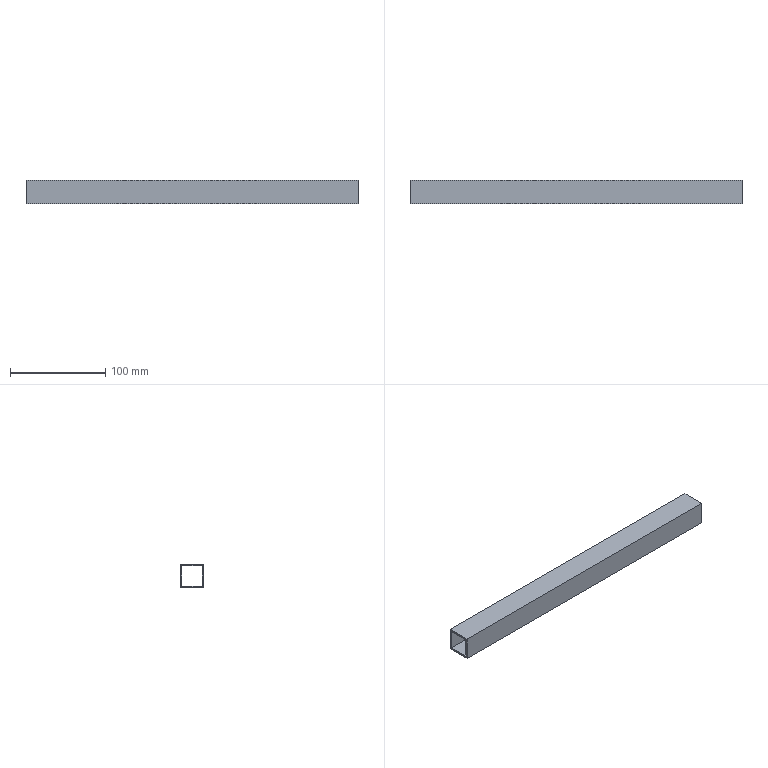Part | NX | features solid 2 | 1 solid | 10 faces | box 348.5 x 25 x 25 mm | volume 64124 mm3 | plane 10
STEP:
#1=CARTESIAN_POINT('',(-348.5,-81.5,-75.));
#2=VERTEX_POINT('',#1);
#3=CARTESIAN_POINT('',(-348.5,-81.5,-50.));
#4=VERTEX_POINT('',#3);
#5=CARTESIAN_POINT('',(-348.5,-81.5,-77.5));
#6=DIRECTION('',(0.,0.,1.));
#7=VECTOR('',#6,1000.);
#8=LINE('',#5,#7);
#9=EDGE_CURVE('',#2,#4,#8,.T.);
#10=ORIENTED_EDGE('',*,*,#9,.T.);
#11=CARTESIAN_POINT('',(0.,-81.5,-50.));
#12=VERTEX_POINT('',#11);
#13=CARTESIAN_POINT('',(-94.,-81.5,-50.));
#14=DIRECTION('',(-1.,0.,0.));
#15=VECTOR('',#14,1000.);
#16=LINE('',#13,#15);
#17=EDGE_CURVE('',#12,#4,#16,.T.);
#18=ORIENTED_EDGE('',*,*,#17,.F.);
#19=CARTESIAN_POINT('',(0.,-81.5,-75.));
#20=VERTEX_POINT('',#19);
#21=CARTESIAN_POINT('',(0.,-81.5,-77.5));
#22=DIRECTION('',(0.,0.,-1.));
#23=VECTOR('',#22,1000.);
#24=LINE('',#21,#23);
#25=EDGE_CURVE('',#12,#20,#24,.T.);
#26=ORIENTED_EDGE('',*,*,#25,.T.);
#27=CARTESIAN_POINT('',(-94.,-81.5,-75.));
#28=DIRECTION('',(-1.,0.,0.));
#29=VECTOR('',#28,1000.);
#30=LINE('',#27,#29);
#31=EDGE_CURVE('',#20,#2,#30,.T.);
#32=ORIENTED_EDGE('',*,*,#31,.T.);
#33=EDGE_LOOP('',(#10,#18,#26,#32));
#34=FACE_BOUND('',#33,.T.);
#35=CARTESIAN_POINT('',(-94.,-81.5,-77.5));
#36=DIRECTION('',(0.,1.,0.));
#37=DIRECTION('',(0.,0.,1.));
#38=AXIS2_PLACEMENT_3D('',#35,#36,#37);
#39=PLANE('',#38);
#40=ADVANCED_FACE('',(#34),#39,.T.);
#41=CARTESIAN_POINT('',(-348.5,-106.5,-50.));
#42=VERTEX_POINT('',#41);
#43=CARTESIAN_POINT('',(-348.5,-79.,-50.));
#44=DIRECTION('',(0.,-1.,0.));
#45=VECTOR('',#44,1000.);
#46=LINE('',#43,#45);
#47=EDGE_CURVE('',#4,#42,#46,.T.);
#48=ORIENTED_EDGE('',*,*,#47,.T.);
#49=CARTESIAN_POINT('',(0.,-106.5,-50.));
#50=VERTEX_POINT('',#49);
#51=CARTESIAN_POINT('',(-94.,-106.5,-50.));
#52=DIRECTION('',(-1.,0.,0.));
#53=VECTOR('',#52,1000.);
#54=LINE('',#51,#53);
#55=EDGE_CURVE('',#50,#42,#54,.T.);
#56=ORIENTED_EDGE('',*,*,#55,.F.);
#57=CARTESIAN_POINT('',(0.,-79.,-50.));
#58=DIRECTION('',(0.,1.,0.));
#59=VECTOR('',#58,1000.);
#60=LINE('',#57,#59);
#61=EDGE_CURVE('',#50,#12,#60,.T.);
#62=ORIENTED_EDGE('',*,*,#61,.T.);
#63=ORIENTED_EDGE('',*,*,#17,.T.);
#64=EDGE_LOOP('',(#48,#56,#62,#63));
#65=FACE_BOUND('',#64,.T.);
#66=CARTESIAN_POINT('',(-94.,-79.,-50.));
#67=DIRECTION('',(0.,0.,1.));
#68=DIRECTION('',(0.,-1.,0.));
#69=AXIS2_PLACEMENT_3D('',#66,#67,#68);
#70=PLANE('',#69);
#71=ADVANCED_FACE('',(#65),#70,.T.);
#72=CARTESIAN_POINT('',(-348.5,-106.5,-75.));
#73=VERTEX_POINT('',#72);
#74=CARTESIAN_POINT('',(-348.5,-106.5,-47.5));
#75=DIRECTION('',(0.,0.,-1.));
#76=VECTOR('',#75,1000.);
#77=LINE('',#74,#76);
#78=EDGE_CURVE('',#42,#73,#77,.T.);
#79=ORIENTED_EDGE('',*,*,#78,.T.);
#80=CARTESIAN_POINT('',(0.,-106.5,-75.));
#81=VERTEX_POINT('',#80);
#82=CARTESIAN_POINT('',(-94.,-106.5,-75.));
#83=DIRECTION('',(-1.,0.,0.));
#84=VECTOR('',#83,1000.);
#85=LINE('',#82,#84);
#86=EDGE_CURVE('',#81,#73,#85,.T.);
#87=ORIENTED_EDGE('',*,*,#86,.F.);
#88=CARTESIAN_POINT('',(0.,-106.5,-47.5));
#89=DIRECTION('',(0.,0.,1.));
#90=VECTOR('',#89,1000.);
#91=LINE('',#88,#90);
#92=EDGE_CURVE('',#81,#50,#91,.T.);
#93=ORIENTED_EDGE('',*,*,#92,.T.);
#94=ORIENTED_EDGE('',*,*,#55,.T.);
#95=EDGE_LOOP('',(#79,#87,#93,#94));
#96=FACE_BOUND('',#95,.T.);
#97=CARTESIAN_POINT('',(-94.,-106.5,-47.5));
#98=DIRECTION('',(0.,-1.,0.));
#99=DIRECTION('',(0.,0.,-1.));
#100=AXIS2_PLACEMENT_3D('',#97,#98,#99);
#101=PLANE('',#100);
#102=ADVANCED_FACE('',(#96),#101,.T.);
#103=CARTESIAN_POINT('',(-348.5,-109.,-75.));
#104=DIRECTION('',(0.,1.,0.));
#105=VECTOR('',#104,1000.);
#106=LINE('',#103,#105);
#107=EDGE_CURVE('',#73,#2,#106,.T.);
#108=ORIENTED_EDGE('',*,*,#107,.T.);
#109=ORIENTED_EDGE('',*,*,#31,.F.);
#110=CARTESIAN_POINT('',(0.,-109.,-75.));
#111=DIRECTION('',(0.,-1.,0.));
#112=VECTOR('',#111,1000.);
#113=LINE('',#110,#112);
#114=EDGE_CURVE('',#20,#81,#113,.T.);
#115=ORIENTED_EDGE('',*,*,#114,.T.);
#116=ORIENTED_EDGE('',*,*,#86,.T.);
#117=EDGE_LOOP('',(#108,#109,#115,#116));
#118=FACE_BOUND('',#117,.T.);
#119=CARTESIAN_POINT('',(-94.,-109.,-75.));
#120=DIRECTION('',(0.,0.,-1.));
#121=DIRECTION('',(0.,1.,0.));
#122=AXIS2_PLACEMENT_3D('',#119,#120,#121);
#123=PLANE('',#122);
#124=ADVANCED_FACE('',(#118),#123,.T.);
#125=ORIENTED_EDGE('',*,*,#25,.F.);
#126=ORIENTED_EDGE('',*,*,#61,.F.);
#127=ORIENTED_EDGE('',*,*,#92,.F.);
#128=ORIENTED_EDGE('',*,*,#114,.F.);
#129=EDGE_LOOP('',(#125,#126,#127,#128));
#130=FACE_BOUND('',#129,.T.);
#131=CARTESIAN_POINT('',(0.,-104.5,-52.));
#132=VERTEX_POINT('',#131);
#133=CARTESIAN_POINT('',(0.,-83.5,-52.));
#134=VERTEX_POINT('',#133);
#135=CARTESIAN_POINT('',(0.,-79.,-52.));
#136=DIRECTION('',(0.,1.,0.));
#137=VECTOR('',#136,1000.);
#138=LINE('',#135,#137);
#139=EDGE_CURVE('',#132,#134,#138,.T.);
#140=ORIENTED_EDGE('',*,*,#139,.T.);
#141=CARTESIAN_POINT('',(0.,-83.5,-73.));
#142=VERTEX_POINT('',#141);
#143=CARTESIAN_POINT('',(0.,-83.5,-77.5));
#144=DIRECTION('',(0.,0.,-1.));
#145=VECTOR('',#144,1000.);
#146=LINE('',#143,#145);
#147=EDGE_CURVE('',#134,#142,#146,.T.);
#148=ORIENTED_EDGE('',*,*,#147,.T.);
#149=CARTESIAN_POINT('',(0.,-104.5,-73.));
#150=VERTEX_POINT('',#149);
#151=CARTESIAN_POINT('',(0.,-109.,-73.));
#152=DIRECTION('',(0.,-1.,0.));
#153=VECTOR('',#152,1000.);
#154=LINE('',#151,#153);
#155=EDGE_CURVE('',#142,#150,#154,.T.);
#156=ORIENTED_EDGE('',*,*,#155,.T.);
#157=CARTESIAN_POINT('',(0.,-104.5,-47.5));
#158=DIRECTION('',(0.,0.,1.));
#159=VECTOR('',#158,1000.);
#160=LINE('',#157,#159);
#161=EDGE_CURVE('',#150,#132,#160,.T.);
#162=ORIENTED_EDGE('',*,*,#161,.T.);
#163=EDGE_LOOP('',(#140,#148,#156,#162));
#164=FACE_BOUND('',#163,.T.);
#165=CARTESIAN_POINT('',(0.,0.,26.5));
#166=DIRECTION('',(-1.,0.,0.));
#167=DIRECTION('',(0.,0.,-1.));
#168=AXIS2_PLACEMENT_3D('',#165,#166,#167);
#169=PLANE('',#168);
#170=ADVANCED_FACE('',(#130,#164),#169,.F.);
#171=CARTESIAN_POINT('',(-348.5,-83.5,-73.));
#172=VERTEX_POINT('',#171);
#173=CARTESIAN_POINT('',(-94.,-83.5,-73.));
#174=DIRECTION('',(-1.,0.,0.));
#175=VECTOR('',#174,1000.);
#176=LINE('',#173,#175);
#177=EDGE_CURVE('',#142,#172,#176,.T.);
#178=ORIENTED_EDGE('',*,*,#177,.F.);
#179=ORIENTED_EDGE('',*,*,#147,.F.);
#180=CARTESIAN_POINT('',(-348.5,-83.5,-52.));
#181=VERTEX_POINT('',#180);
#182=CARTESIAN_POINT('',(-94.,-83.5,-52.));
#183=DIRECTION('',(-1.,0.,0.));
#184=VECTOR('',#183,1000.);
#185=LINE('',#182,#184);
#186=EDGE_CURVE('',#134,#181,#185,.T.);
#187=ORIENTED_EDGE('',*,*,#186,.T.);
#188=CARTESIAN_POINT('',(-348.5,-83.5,-77.5));
#189=DIRECTION('',(0.,0.,1.));
#190=VECTOR('',#189,1000.);
#191=LINE('',#188,#190);
#192=EDGE_CURVE('',#172,#181,#191,.T.);
#193=ORIENTED_EDGE('',*,*,#192,.F.);
#194=EDGE_LOOP('',(#178,#179,#187,#193));
#195=FACE_BOUND('',#194,.T.);
#196=CARTESIAN_POINT('',(-94.,-83.5,-77.5));
#197=DIRECTION('',(0.,1.,0.));
#198=DIRECTION('',(0.,0.,1.));
#199=AXIS2_PLACEMENT_3D('',#196,#197,#198);
#200=PLANE('',#199);
#201=ADVANCED_FACE('',(#195),#200,.F.);
#202=ORIENTED_EDGE('',*,*,#186,.F.);
#203=ORIENTED_EDGE('',*,*,#139,.F.);
#204=CARTESIAN_POINT('',(-348.5,-104.5,-52.));
#205=VERTEX_POINT('',#204);
#206=CARTESIAN_POINT('',(-94.,-104.5,-52.));
#207=DIRECTION('',(-1.,0.,0.));
#208=VECTOR('',#207,1000.);
#209=LINE('',#206,#208);
#210=EDGE_CURVE('',#132,#205,#209,.T.);
#211=ORIENTED_EDGE('',*,*,#210,.T.);
#212=CARTESIAN_POINT('',(-348.5,-79.,-52.));
#213=DIRECTION('',(0.,-1.,0.));
#214=VECTOR('',#213,1000.);
#215=LINE('',#212,#214);
#216=EDGE_CURVE('',#181,#205,#215,.T.);
#217=ORIENTED_EDGE('',*,*,#216,.F.);
#218=EDGE_LOOP('',(#202,#203,#211,#217));
#219=FACE_BOUND('',#218,.T.);
#220=CARTESIAN_POINT('',(-94.,-79.,-52.));
#221=DIRECTION('',(0.,0.,1.));
#222=DIRECTION('',(0.,-1.,0.));
#223=AXIS2_PLACEMENT_3D('',#220,#221,#222);
#224=PLANE('',#223);
#225=ADVANCED_FACE('',(#219),#224,.F.);
#226=ORIENTED_EDGE('',*,*,#210,.F.);
#227=ORIENTED_EDGE('',*,*,#161,.F.);
#228=CARTESIAN_POINT('',(-348.5,-104.5,-73.));
#229=VERTEX_POINT('',#228);
#230=CARTESIAN_POINT('',(-94.,-104.5,-73.));
#231=DIRECTION('',(-1.,0.,0.));
#232=VECTOR('',#231,1000.);
#233=LINE('',#230,#232);
#234=EDGE_CURVE('',#150,#229,#233,.T.);
#235=ORIENTED_EDGE('',*,*,#234,.T.);
#236=CARTESIAN_POINT('',(-348.5,-104.5,-47.5));
#237=DIRECTION('',(0.,0.,-1.));
#238=VECTOR('',#237,1000.);
#239=LINE('',#236,#238);
#240=EDGE_CURVE('',#205,#229,#239,.T.);
#241=ORIENTED_EDGE('',*,*,#240,.F.);
#242=EDGE_LOOP('',(#226,#227,#235,#241));
#243=FACE_BOUND('',#242,.T.);
#244=CARTESIAN_POINT('',(-94.,-104.5,-47.5));
#245=DIRECTION('',(0.,-1.,0.));
#246=DIRECTION('',(0.,0.,-1.));
#247=AXIS2_PLACEMENT_3D('',#244,#245,#246);
#248=PLANE('',#247);
#249=ADVANCED_FACE('',(#243),#248,.F.);
#250=ORIENTED_EDGE('',*,*,#234,.F.);
#251=ORIENTED_EDGE('',*,*,#155,.F.);
#252=ORIENTED_EDGE('',*,*,#177,.T.);
#253=CARTESIAN_POINT('',(-348.5,-109.,-73.));
#254=DIRECTION('',(0.,1.,0.));
#255=VECTOR('',#254,1000.);
#256=LINE('',#253,#255);
#257=EDGE_CURVE('',#229,#172,#256,.T.);
#258=ORIENTED_EDGE('',*,*,#257,.F.);
#259=EDGE_LOOP('',(#250,#251,#252,#258));
#260=FACE_BOUND('',#259,.T.);
#261=CARTESIAN_POINT('',(-94.,-109.,-73.));
#262=DIRECTION('',(0.,0.,-1.));
#263=DIRECTION('',(0.,1.,0.));
#264=AXIS2_PLACEMENT_3D('',#261,#262,#263);
#265=PLANE('',#264);
#266=ADVANCED_FACE('',(#260),#265,.F.);
#267=ORIENTED_EDGE('',*,*,#107,.F.);
#268=ORIENTED_EDGE('',*,*,#78,.F.);
#269=ORIENTED_EDGE('',*,*,#47,.F.);
#270=ORIENTED_EDGE('',*,*,#9,.F.);
#271=EDGE_LOOP('',(#267,#268,#269,#270));
#272=FACE_BOUND('',#271,.T.);
#273=ORIENTED_EDGE('',*,*,#240,.T.);
#274=ORIENTED_EDGE('',*,*,#257,.T.);
#275=ORIENTED_EDGE('',*,*,#192,.T.);
#276=ORIENTED_EDGE('',*,*,#216,.T.);
#277=EDGE_LOOP('',(#273,#274,#275,#276));
#278=FACE_BOUND('',#277,.T.);
#279=CARTESIAN_POINT('',(-348.5,-227.,-75.));
#280=DIRECTION('',(1.,0.,0.));
#281=DIRECTION('',(0.,0.,1.));
#282=AXIS2_PLACEMENT_3D('',#279,#280,#281);
#283=PLANE('',#282);
#284=ADVANCED_FACE('',(#272,#278),#283,.F.);
#285=CLOSED_SHELL('',(#40,#71,#102,#124,#170,#201,#225,#249,#266,#284));
#286=MANIFOLD_SOLID_BREP('',#285);
#287=(LENGTH_UNIT()NAMED_UNIT(*)SI_UNIT(.MILLI.,.METRE.));
#288=UNCERTAINTY_MEASURE_WITH_UNIT(LENGTH_MEASURE(0.00001),#287,'','');
#289=(NAMED_UNIT(*)PLANE_ANGLE_UNIT()SI_UNIT($,.RADIAN.));
#290=(NAMED_UNIT(*)SI_UNIT($,.STERADIAN.)SOLID_ANGLE_UNIT());
#291=(GEOMETRIC_REPRESENTATION_CONTEXT(3)GLOBAL_UNCERTAINTY_ASSIGNED_CONTEXT((#288))GLOBAL_UNIT_ASSIGNED_CONTEXT((#287,#289,#290))REPRESENTATION_CONTEXT('',''));
#292=ADVANCED_BREP_SHAPE_REPRESENTATION('',(#286),#291);